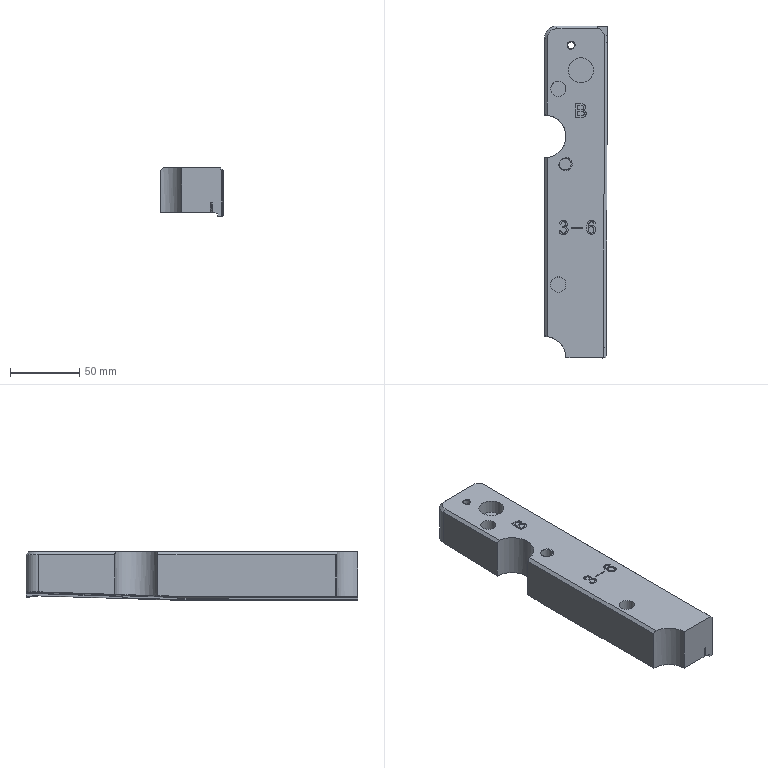NC program | NX | posted with a generic post | part box 45.476 x 239.737 x 35.001 mm
Lines 1 to 136 of 14047:
N10 G17 G21 G94 G90
(FACE_MILLING_COPY , TOOL : D8)
N12 T00 M6
N14 G53
N16 G17 G0 G90 X122.583 Y-5.453 S4500 M3
N18 G43 Z60. H0
N20 G94 G1 Z29.232 F4000.
N22 Z29.032 F600.
N24 Y-10.253
N26 Y-19.376 F1000.
N28 G2 X117.783 Y-24.747 R13.
N30 G1 Y-10.253
N32 X112.983
N34 Y-26.565
N36 Y-31.365
N38 Z29.232
N40 G0 Z60.
N42 X128.669 Y1.63
N44 G1 Z10.2 F4000.
N46 Z10. F600.
N48 X123.869
N50 X92.438 F1000.
N52 G2 X93.189 Y0.644 R22.9
N54 G1 X123.869
N56 Y-4.156
N58 X90.542
N60 G3 X85.023 Y2.064 R18.1
N62 G1 Y6.43
N64 X123.869
N66 Y11.23
N68 X81.166
N70 G3 X80.223 Y10.376 R0.839
N72 G1 X80.244 Y-0.692
N74 G2 X87.357 Y-8.956 R13.3
N76 G1 X123.869
N78 X128.669
N80 Z10.2
N82 G0 Z60.
N84 X89.566 Y-4.627
N86 G1 Z19.2 F4000.
N88 Z19. F600.
N90 X84.766
N92 X84.525 F1000.
N94 X84.23 Y-4.671
N96 X84.314 Y-4.092
N98 G3 X79.752 Y-0.8 R13.
N100 G1 Y-2.109
N102 X79.546 Y-3.529
N104 G2 X74.112 Y-8.064 R6.256
N106 G3 X79.129 Y-14.017 R-4.7
N108 G1 X79.204 Y-13.752
N110 X79.349 Y-13.412
N112 X74.713 Y-12.648
N114 X79.349 Y-13.412
N116 X79.692 Y-12.607
N118 X80.578 Y-11.388
N120 X81.818 Y-10.358
N122 X83.416 Y-9.643
N124 X84.877 Y-9.427
N126 X87.177
N128 X91.977
N130 Y-8.427
N132 Z19.2
N134 G0 Z60.
N136 X-113.169 Y-22.922
N138 G1 Z32.419 F4000.
N140 Z32.219 F600.
N142 X-108.369 Y-22.901
N144 X-31.003 Y-22.563 F1000.
N146 X10.76 Y-22.114
N148 G3 X11.309 Y-22.105 R158.513
N150 G1 Y-17.304
N152 G2 X10.694 Y-17.315 R153.713
N154 G1 X-31.039 Y-17.763
N156 X-109.343 Y-18.105
N158 G3 X-113.267 Y-13.322 R11.5
N160 G1 X-31.075 Y-12.963
N162 X10.629 Y-12.515
N164 G3 X11.309 Y-12.502 R148.913
N166 G1 Y-7.701
N168 G2 X10.563 Y-7.716 R144.113
N170 G1 X-31.111 Y-8.163
N172 X-123.785 Y-8.568
N174 X-123.869
N176 Y-3.768
N178 X-123.806
N180 X-31.132 Y-3.363
N182 X10.497 Y-2.916
N184 G3 X11.309 Y-2.9 R139.313
N186 G1 Y1.901
N188 G2 X10.43 Y1.883 R134.513
N190 G1 X-31.152 Y1.437
N192 X-123.827 Y1.032
N194 X-123.869
N196 Y5.832
N198 X-123.848
N200 X-31.173 Y6.237
N202 X10.364 Y6.683
N204 G3 X11.309 Y6.702 R129.713
N206 G1 Y11.504
N208 G2 X10.296 Y11.482 R124.913
N210 G1 X-30.152 Y11.041
N212 X-31.194 Y11.037
N214 X-123.869 Y10.632
N216 X-128.669 Y10.611
N218 Z32.419
N220 G0 Z60.
N222 X-54.876 Y30.773
N224 G1 Z35.201 F4000.
N226 Z35.001 F600.
N228 X-54.853 Y25.973
N230 X14.207 Y26.298 F1000.
N232 Y16.026
N234 X10.247 Y16.025
N236 X10.203 Y16.024
N238 X-31.333 Y15.513
N240 X-123.869 Y14.999
N242 Y25.641
N244 X-108.131 Y25.725
N246 X-54.853 Y25.973
N248 X-54.831 Y21.173
N250 X9.407 Y21.475
N252 Y20.815
N254 X-26.992 Y20.36
N256 X-27.379 Y20.335
N258 X-119.069 Y19.826
N260 Y20.866
N262 X-54.831 Y21.173
N264 X-54.858 Y26.973
N266 Z35.201
N268 G0 Z60.
N270 M5